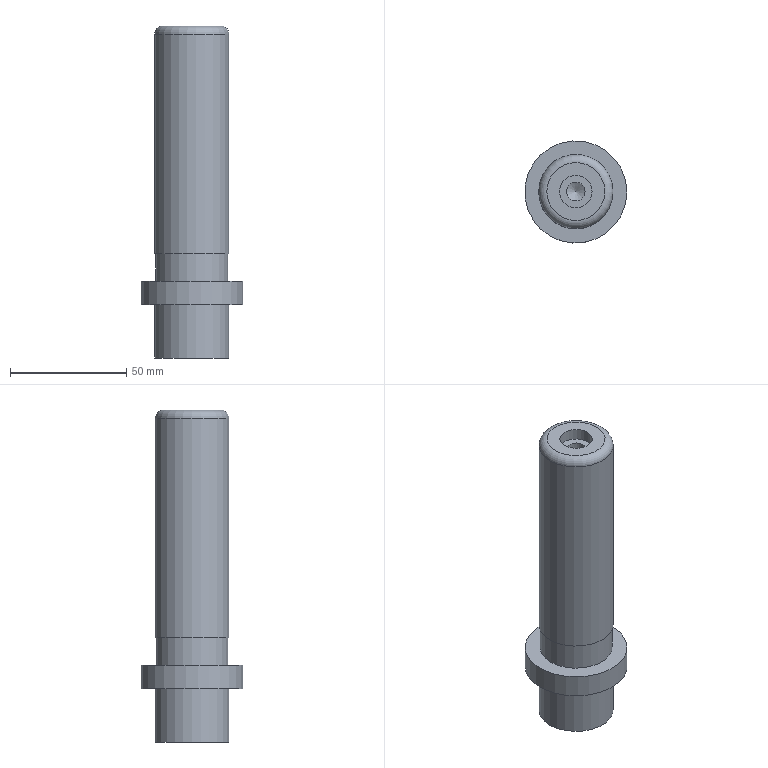Part | STEP file | 1_id1574_x_t | 1 solid | 147 faces | box 44 x 44 x 143 mm | volume 118157 mm3 | plane 73 | other 62 | cylinder 8 | cone 3 | torus 1 | commonest cylinder face diameters 32 x2 8 x1 8.5 x1 10 x1 14 x1 31 x1